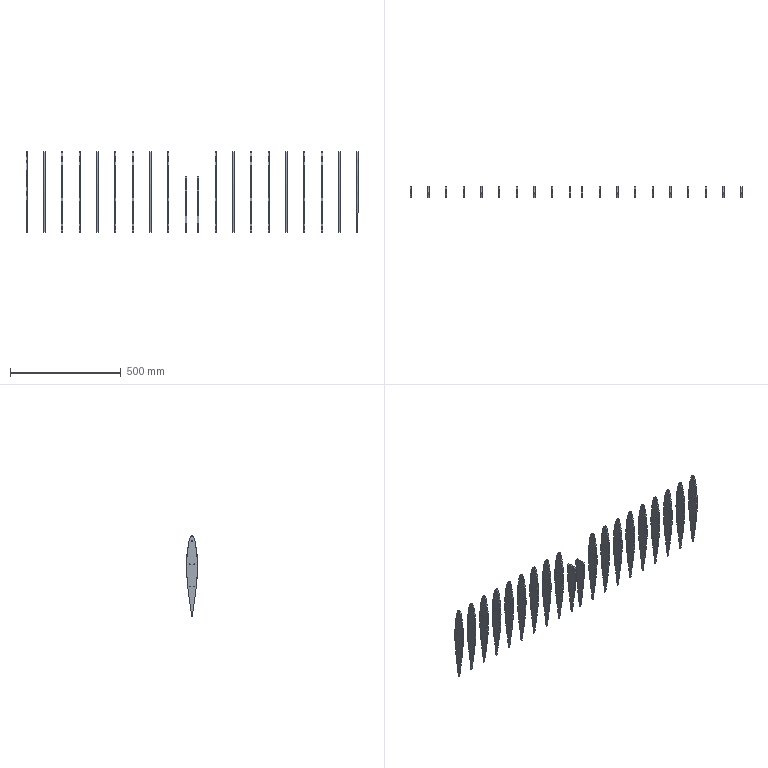Part | SolidWorks | features BaseBody 20 | 20 solids | 520 faces | box 1500 x 50.063 x 363.99 mm | volume 828337 mm3 | plane 302 | cylinder 196 | spline 22 | commonest cylinder face diameters 4 x196